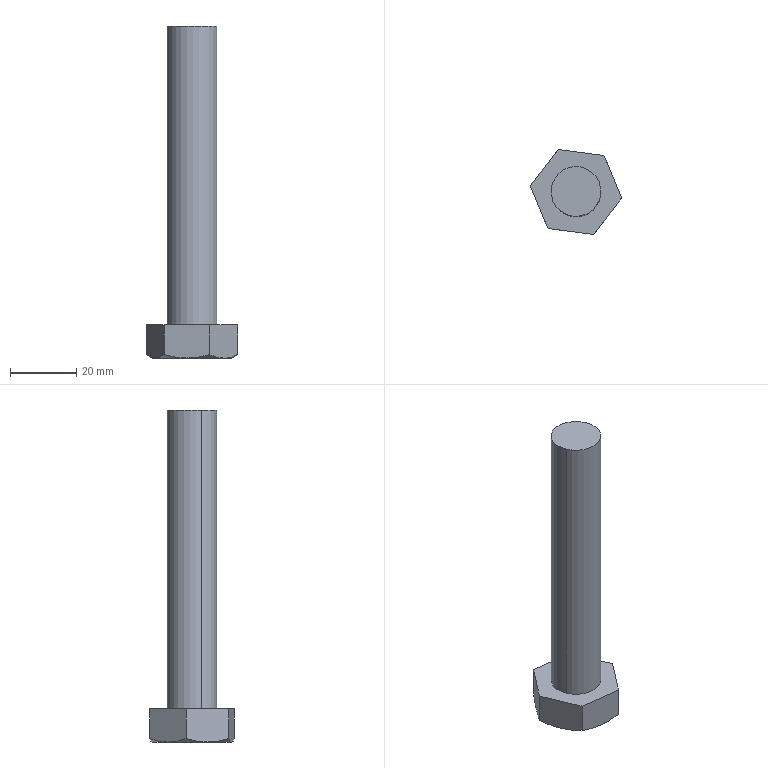Part | SolidWorks | features BaseBody 1 | 1 solid | 17 faces | box 27.477 x 25.599 x 100 mm | volume 20878 mm3 | plane 9 | cone 6 | cylinder 2 | commonest cylinder face diameters 15 x2
STEP:
#1=CARTESIAN_POINT('',(263.515,1086.351,-654.893));
#2=VERTEX_POINT('',#1);
#3=CARTESIAN_POINT('',(253.992,1093.652,-654.893));
#4=VERTEX_POINT('',#3);
#5=CARTESIAN_POINT('',(265.077,1098.249,-654.893));
#6=DIRECTION('',(0.,0.,-1.));
#7=DIRECTION('',(-0.9237,-0.383,0.));
#8=AXIS2_PLACEMENT_3D('',#5,#6,#7);
#9=CIRCLE('',#8,12.);
#10=EDGE_CURVE('',#2,#4,#9,.T.);
#11=ORIENTED_EDGE('',*,*,#10,.T.);
#12=CARTESIAN_POINT('',(255.554,1105.55,-654.893));
#13=VERTEX_POINT('',#12);
#14=CARTESIAN_POINT('',(265.077,1098.249,-654.893));
#15=DIRECTION('',(0.,0.,-1.));
#16=DIRECTION('',(-0.9237,-0.383,0.));
#17=AXIS2_PLACEMENT_3D('',#14,#15,#16);
#18=CIRCLE('',#17,12.);
#19=EDGE_CURVE('',#4,#13,#18,.T.);
#20=ORIENTED_EDGE('',*,*,#19,.T.);
#21=CARTESIAN_POINT('',(266.639,1110.147,-654.893));
#22=VERTEX_POINT('',#21);
#23=CARTESIAN_POINT('',(265.077,1098.249,-654.893));
#24=DIRECTION('',(0.,0.,-1.));
#25=DIRECTION('',(-0.9237,-0.383,0.));
#26=AXIS2_PLACEMENT_3D('',#23,#24,#25);
#27=CIRCLE('',#26,12.);
#28=EDGE_CURVE('',#13,#22,#27,.T.);
#29=ORIENTED_EDGE('',*,*,#28,.T.);
#30=CARTESIAN_POINT('',(276.162,1102.846,-654.893));
#31=VERTEX_POINT('',#30);
#32=CARTESIAN_POINT('',(265.077,1098.249,-654.893));
#33=DIRECTION('',(0.,0.,-1.));
#34=DIRECTION('',(-0.9237,-0.383,0.));
#35=AXIS2_PLACEMENT_3D('',#32,#33,#34);
#36=CIRCLE('',#35,12.);
#37=EDGE_CURVE('',#22,#31,#36,.T.);
#38=ORIENTED_EDGE('',*,*,#37,.T.);
#39=CARTESIAN_POINT('',(274.6,1090.948,-654.893));
#40=VERTEX_POINT('',#39);
#41=CARTESIAN_POINT('',(265.077,1098.249,-654.893));
#42=DIRECTION('',(0.,0.,-1.));
#43=DIRECTION('',(-0.9237,-0.383,0.));
#44=AXIS2_PLACEMENT_3D('',#41,#42,#43);
#45=CIRCLE('',#44,12.);
#46=EDGE_CURVE('',#31,#40,#45,.T.);
#47=ORIENTED_EDGE('',*,*,#46,.T.);
#48=CARTESIAN_POINT('',(265.077,1098.249,-654.893));
#49=DIRECTION('',(0.,0.,-1.));
#50=DIRECTION('',(-0.9237,-0.383,0.));
#51=AXIS2_PLACEMENT_3D('',#48,#49,#50);
#52=CIRCLE('',#51,12.);
#53=EDGE_CURVE('',#40,#2,#52,.T.);
#54=ORIENTED_EDGE('',*,*,#53,.T.);
#55=EDGE_LOOP('',(#11,#20,#29,#38,#47,#54));
#56=FACE_OUTER_BOUND('',#55,.T.);
#57=CARTESIAN_POINT('',(259.769,1111.048,-654.893));
#58=DIRECTION('',(0.,0.,-1.));
#59=DIRECTION('',(0.,-1.,0.));
#60=AXIS2_PLACEMENT_3D('',#57,#58,#59);
#61=PLANE('',#60);
#62=ADVANCED_FACE('',(#56),#61,.T.);
#63=CARTESIAN_POINT('',(251.338,1100.052,-653.822));
#64=VERTEX_POINT('',#63);
#65=CARTESIAN_POINT('',(251.338,1100.052,-653.822));
#66=CARTESIAN_POINT('',(251.697,1100.52,-653.992));
#67=CARTESIAN_POINT('',(252.049,1100.978,-654.142));
#68=CARTESIAN_POINT('',(252.568,1101.655,-654.338));
#69=CARTESIAN_POINT('',(252.74,1101.88,-654.398));
#70=CARTESIAN_POINT('',(252.996,1102.215,-654.481));
#71=CARTESIAN_POINT('',(253.125,1102.382,-654.521));
#72=CARTESIAN_POINT('',(253.274,1102.576,-654.564));
#73=CARTESIAN_POINT('',(253.338,1102.66,-654.581));
#74=CARTESIAN_POINT('',(253.38,1102.715,-654.593));
#75=CARTESIAN_POINT('',(253.401,1102.742,-654.598));
#76=CARTESIAN_POINT('',(253.601,1103.003,-654.652));
#77=CARTESIAN_POINT('',(253.777,1103.233,-654.693));
#78=CARTESIAN_POINT('',(254.042,1103.578,-654.747));
#79=CARTESIAN_POINT('',(254.174,1103.75,-654.771));
#80=CARTESIAN_POINT('',(254.306,1103.922,-654.793));
#81=CARTESIAN_POINT('',(254.394,1104.037,-654.806));
#82=CARTESIAN_POINT('',(254.437,1104.093,-654.813));
#83=CARTESIAN_POINT('',(254.841,1104.621,-654.869));
#84=CARTESIAN_POINT('',(255.196,1105.084,-654.893));
#85=CARTESIAN_POINT('',(255.554,1105.55,-654.893));
#86=B_SPLINE_CURVE_WITH_KNOTS('',3,(#65,#66,#67,#68,#69,#70,#71,#72,#73,#74,#75,#76,#77,#78,#79,#80,#81,#82,#83,#84,#85),.UNSPECIFIED.,.F.,.F.,(4,2,2,1,1,2,2,2,1,2,2,4),(0.,0.25,0.375,0.4375,0.4688,0.4844,0.5,0.625,0.6875,0.7188,0.75,1.),.UNSPECIFIED.);
#87=EDGE_CURVE('',#64,#13,#86,.T.);
#88=ORIENTED_EDGE('',*,*,#87,.T.);
#89=ORIENTED_EDGE('',*,*,#19,.F.);
#90=CARTESIAN_POINT('',(253.992,1093.652,-654.893));
#91=CARTESIAN_POINT('',(253.88,1093.924,-654.893));
#92=CARTESIAN_POINT('',(253.767,1094.194,-654.887));
#93=CARTESIAN_POINT('',(253.599,1094.6,-654.869));
#94=CARTESIAN_POINT('',(253.543,1094.736,-654.861));
#95=CARTESIAN_POINT('',(253.458,1094.94,-654.847));
#96=CARTESIAN_POINT('',(253.43,1095.007,-654.842));
#97=CARTESIAN_POINT('',(253.374,1095.144,-654.831));
#98=CARTESIAN_POINT('',(253.345,1095.213,-654.825));
#99=CARTESIAN_POINT('',(253.206,1095.547,-654.795));
#100=CARTESIAN_POINT('',(253.096,1095.814,-654.765));
#101=CARTESIAN_POINT('',(252.929,1096.215,-654.711));
#102=CARTESIAN_POINT('',(252.846,1096.416,-654.682));
#103=CARTESIAN_POINT('',(252.748,1096.652,-654.644));
#104=CARTESIAN_POINT('',(252.707,1096.753,-654.627));
#105=CARTESIAN_POINT('',(252.679,1096.82,-654.616));
#106=CARTESIAN_POINT('',(252.664,1096.855,-654.61));
#107=CARTESIAN_POINT('',(252.222,1097.922,-654.423));
#108=CARTESIAN_POINT('',(251.79,1098.962,-654.162));
#109=CARTESIAN_POINT('',(251.338,1100.052,-653.822));
#110=B_SPLINE_CURVE_WITH_KNOTS('',3,(#90,#91,#92,#93,#94,#95,#96,#97,#98,#99,#100,#101,#102,#103,#104,#105,#106,#107,#108,#109),.UNSPECIFIED.,.F.,.F.,(4,2,2,2,2,2,1,1,2,2,4),(0.,0.125,0.1875,0.2188,0.25,0.375,0.4375,0.4688,0.4844,0.5,1.),.UNSPECIFIED.);
#111=EDGE_CURVE('',#4,#64,#110,.T.);
#112=ORIENTED_EDGE('',*,*,#111,.T.);
#113=EDGE_LOOP('',(#88,#89,#112));
#114=FACE_OUTER_BOUND('',#113,.T.);
#115=CARTESIAN_POINT('',(265.077,1098.249,-654.893));
#116=DIRECTION('',(0.,0.,1.));
#117=DIRECTION('',(0.9237,0.383,0.));
#118=AXIS2_PLACEMENT_3D('',#115,#116,#117);
#119=CONICAL_SURFACE('',#118,12.,1.047);
#120=ADVANCED_FACE('',(#114),#119,.T.);
#121=CARTESIAN_POINT('',(259.769,1111.048,-653.822));
#122=VERTEX_POINT('',#121);
#123=CARTESIAN_POINT('',(255.554,1105.55,-654.893));
#124=CARTESIAN_POINT('',(255.733,1105.784,-654.893));
#125=CARTESIAN_POINT('',(255.911,1106.016,-654.887));
#126=CARTESIAN_POINT('',(256.178,1106.365,-654.869));
#127=CARTESIAN_POINT('',(256.312,1106.539,-654.857));
#128=CARTESIAN_POINT('',(256.446,1106.715,-654.842));
#129=CARTESIAN_POINT('',(256.536,1106.832,-654.831));
#130=CARTESIAN_POINT('',(256.582,1106.891,-654.825));
#131=CARTESIAN_POINT('',(256.802,1107.178,-654.795));
#132=CARTESIAN_POINT('',(256.978,1107.408,-654.765));
#133=CARTESIAN_POINT('',(257.242,1107.752,-654.711));
#134=CARTESIAN_POINT('',(257.374,1107.925,-654.682));
#135=CARTESIAN_POINT('',(257.529,1108.127,-654.644));
#136=CARTESIAN_POINT('',(257.596,1108.214,-654.627));
#137=CARTESIAN_POINT('',(257.64,1108.272,-654.616));
#138=CARTESIAN_POINT('',(257.663,1108.302,-654.61));
#139=CARTESIAN_POINT('',(258.366,1109.218,-654.423));
#140=CARTESIAN_POINT('',(259.051,1110.112,-654.162));
#141=CARTESIAN_POINT('',(259.769,1111.048,-653.822));
#142=B_SPLINE_CURVE_WITH_KNOTS('',3,(#123,#124,#125,#126,#127,#128,#129,#130,#131,#132,#133,#134,#135,#136,#137,#138,#139,#140,#141),.UNSPECIFIED.,.F.,.F.,(4,2,1,2,2,2,1,1,2,2,4),(0.,0.125,0.1875,0.2187,0.25,0.375,0.4375,0.4687,0.4844,0.5,1.),.UNSPECIFIED.);
#143=EDGE_CURVE('',#13,#122,#142,.T.);
#144=ORIENTED_EDGE('',*,*,#143,.T.);
#145=CARTESIAN_POINT('',(259.769,1111.048,-653.822));
#146=CARTESIAN_POINT('',(260.354,1110.972,-653.992));
#147=CARTESIAN_POINT('',(260.926,1110.896,-654.142));
#148=CARTESIAN_POINT('',(261.773,1110.785,-654.338));
#149=CARTESIAN_POINT('',(262.053,1110.749,-654.398));
#150=CARTESIAN_POINT('',(262.471,1110.694,-654.481));
#151=CARTESIAN_POINT('',(262.68,1110.666,-654.521));
#152=CARTESIAN_POINT('',(262.923,1110.635,-654.564));
#153=CARTESIAN_POINT('',(263.027,1110.621,-654.581));
#154=CARTESIAN_POINT('',(263.097,1110.612,-654.593));
#155=CARTESIAN_POINT('',(263.13,1110.607,-654.598));
#156=CARTESIAN_POINT('',(263.456,1110.565,-654.652));
#157=CARTESIAN_POINT('',(263.744,1110.527,-654.693));
#158=CARTESIAN_POINT('',(264.175,1110.47,-654.747));
#159=CARTESIAN_POINT('',(264.318,1110.452,-654.763));
#160=CARTESIAN_POINT('',(264.533,1110.423,-654.786));
#161=CARTESIAN_POINT('',(264.605,1110.414,-654.793));
#162=CARTESIAN_POINT('',(264.748,1110.395,-654.806));
#163=CARTESIAN_POINT('',(264.818,1110.386,-654.813));
#164=CARTESIAN_POINT('',(265.477,1110.299,-654.869));
#165=CARTESIAN_POINT('',(266.056,1110.223,-654.893));
#166=CARTESIAN_POINT('',(266.639,1110.147,-654.893));
#167=B_SPLINE_CURVE_WITH_KNOTS('',3,(#145,#146,#147,#148,#149,#150,#151,#152,#153,#154,#155,#156,#157,#158,#159,#160,#161,#162,#163,#164,#165,#166),.UNSPECIFIED.,.F.,.F.,(4,2,2,1,1,2,2,2,2,2,2,4),(0.,0.25,0.375,0.4375,0.4688,0.4844,0.5,0.625,0.6875,0.7188,0.75,1.),.UNSPECIFIED.);
#168=EDGE_CURVE('',#122,#22,#167,.T.);
#169=ORIENTED_EDGE('',*,*,#168,.T.);
#170=ORIENTED_EDGE('',*,*,#28,.F.);
#171=EDGE_LOOP('',(#144,#169,#170));
#172=FACE_OUTER_BOUND('',#171,.T.);
#173=CARTESIAN_POINT('',(265.077,1098.249,-654.893));
#174=DIRECTION('',(0.,0.,1.));
#175=DIRECTION('',(0.9237,0.383,0.));
#176=AXIS2_PLACEMENT_3D('',#173,#174,#175);
#177=CONICAL_SURFACE('',#176,12.,1.047);
#178=ADVANCED_FACE('',(#172),#177,.T.);
#179=CARTESIAN_POINT('',(273.508,1109.245,-653.822));
#180=VERTEX_POINT('',#179);
#181=CARTESIAN_POINT('',(266.639,1110.147,-654.893));
#182=CARTESIAN_POINT('',(266.93,1110.109,-654.893));
#183=CARTESIAN_POINT('',(267.22,1110.071,-654.887));
#184=CARTESIAN_POINT('',(267.656,1110.013,-654.869));
#185=CARTESIAN_POINT('',(267.802,1109.994,-654.861));
#186=CARTESIAN_POINT('',(268.02,1109.966,-654.847));
#187=CARTESIAN_POINT('',(268.093,1109.956,-654.842));
#188=CARTESIAN_POINT('',(268.239,1109.937,-654.831));
#189=CARTESIAN_POINT('',(268.314,1109.927,-654.825));
#190=CARTESIAN_POINT('',(268.672,1109.88,-654.795));
#191=CARTESIAN_POINT('',(268.959,1109.842,-654.765));
#192=CARTESIAN_POINT('',(269.39,1109.786,-654.711));
#193=CARTESIAN_POINT('',(269.605,1109.758,-654.682));
#194=CARTESIAN_POINT('',(269.858,1109.724,-654.644));
#195=CARTESIAN_POINT('',(269.966,1109.71,-654.627));
#196=CARTESIAN_POINT('',(270.039,1109.701,-654.616));
#197=CARTESIAN_POINT('',(270.076,1109.696,-654.61));
#198=CARTESIAN_POINT('',(271.221,1109.545,-654.423));
#199=CARTESIAN_POINT('',(272.338,1109.399,-654.162));
#200=CARTESIAN_POINT('',(273.508,1109.245,-653.822));
#201=B_SPLINE_CURVE_WITH_KNOTS('',3,(#181,#182,#183,#184,#185,#186,#187,#188,#189,#190,#191,#192,#193,#194,#195,#196,#197,#198,#199,#200),.UNSPECIFIED.,.F.,.F.,(4,2,2,2,2,2,1,1,2,2,4),(0.,0.125,0.1875,0.2187,0.25,0.375,0.4375,0.4687,0.4844,0.5,1.),.UNSPECIFIED.);
#202=EDGE_CURVE('',#22,#180,#201,.T.);
#203=ORIENTED_EDGE('',*,*,#202,.T.);
#204=CARTESIAN_POINT('',(273.508,1109.245,-653.822));
#205=CARTESIAN_POINT('',(273.734,1108.7,-653.992));
#206=CARTESIAN_POINT('',(273.955,1108.167,-654.142));
#207=CARTESIAN_POINT('',(274.281,1107.379,-654.338));
#208=CARTESIAN_POINT('',(274.39,1107.118,-654.398));
#209=CARTESIAN_POINT('',(274.552,1106.728,-654.481));
#210=CARTESIAN_POINT('',(274.632,1106.534,-654.521));
#211=CARTESIAN_POINT('',(274.726,1106.307,-654.564));
#212=CARTESIAN_POINT('',(274.766,1106.21,-654.581));
#213=CARTESIAN_POINT('',(274.793,1106.145,-654.593));
#214=CARTESIAN_POINT('',(274.806,1106.114,-654.598));
#215=CARTESIAN_POINT('',(274.932,1105.811,-654.652));
#216=CARTESIAN_POINT('',(275.043,1105.542,-654.693));
#217=CARTESIAN_POINT('',(275.21,1105.141,-654.747));
#218=CARTESIAN_POINT('',(275.293,1104.941,-654.771));
#219=CARTESIAN_POINT('',(275.376,1104.74,-654.793));
#220=CARTESIAN_POINT('',(275.431,1104.607,-654.806));
#221=CARTESIAN_POINT('',(275.459,1104.541,-654.813));
#222=CARTESIAN_POINT('',(275.713,1103.927,-654.869));
#223=CARTESIAN_POINT('',(275.936,1103.388,-654.893));
#224=CARTESIAN_POINT('',(276.162,1102.846,-654.893));
#225=B_SPLINE_CURVE_WITH_KNOTS('',3,(#204,#205,#206,#207,#208,#209,#210,#211,#212,#213,#214,#215,#216,#217,#218,#219,#220,#221,#222,#223,#224),.UNSPECIFIED.,.F.,.F.,(4,2,2,1,1,2,2,2,1,2,2,4),(0.,0.25,0.375,0.4375,0.4688,0.4844,0.5,0.625,0.6875,0.7188,0.75,1.),.UNSPECIFIED.);
#226=EDGE_CURVE('',#180,#31,#225,.T.);
#227=ORIENTED_EDGE('',*,*,#226,.T.);
#228=ORIENTED_EDGE('',*,*,#37,.F.);
#229=EDGE_LOOP('',(#203,#227,#228));
#230=FACE_OUTER_BOUND('',#229,.T.);
#231=CARTESIAN_POINT('',(265.077,1098.249,-654.893));
#232=DIRECTION('',(0.,0.,1.));
#233=DIRECTION('',(0.9237,0.383,0.));
#234=AXIS2_PLACEMENT_3D('',#231,#232,#233);
#235=CONICAL_SURFACE('',#234,12.,1.047);
#236=ADVANCED_FACE('',(#230),#235,.T.);
#237=CARTESIAN_POINT('',(278.815,1096.446,-653.822));
#238=VERTEX_POINT('',#237);
#239=CARTESIAN_POINT('',(276.162,1102.846,-654.893));
#240=CARTESIAN_POINT('',(276.274,1102.574,-654.893));
#241=CARTESIAN_POINT('',(276.386,1102.304,-654.887));
#242=CARTESIAN_POINT('',(276.555,1101.897,-654.869));
#243=CARTESIAN_POINT('',(276.611,1101.762,-654.861));
#244=CARTESIAN_POINT('',(276.695,1101.558,-654.847));
#245=CARTESIAN_POINT('',(276.724,1101.49,-654.842));
#246=CARTESIAN_POINT('',(276.78,1101.354,-654.831));
#247=CARTESIAN_POINT('',(276.809,1101.285,-654.825));
#248=CARTESIAN_POINT('',(276.948,1100.951,-654.795));
#249=CARTESIAN_POINT('',(277.058,1100.684,-654.765));
#250=CARTESIAN_POINT('',(277.224,1100.282,-654.711));
#251=CARTESIAN_POINT('',(277.308,1100.082,-654.682));
#252=CARTESIAN_POINT('',(277.405,1099.846,-654.644));
#253=CARTESIAN_POINT('',(277.447,1099.745,-654.627));
#254=CARTESIAN_POINT('',(277.475,1099.678,-654.616));
#255=CARTESIAN_POINT('',(277.49,1099.643,-654.61));
#256=CARTESIAN_POINT('',(277.932,1098.576,-654.423));
#257=CARTESIAN_POINT('',(278.363,1097.536,-654.162));
#258=CARTESIAN_POINT('',(278.815,1096.446,-653.822));
#259=B_SPLINE_CURVE_WITH_KNOTS('',3,(#239,#240,#241,#242,#243,#244,#245,#246,#247,#248,#249,#250,#251,#252,#253,#254,#255,#256,#257,#258),.UNSPECIFIED.,.F.,.F.,(4,2,2,2,2,2,1,1,2,2,4),(0.,0.125,0.1875,0.2188,0.25,0.375,0.4375,0.4688,0.4844,0.5,1.),.UNSPECIFIED.);
#260=EDGE_CURVE('',#31,#238,#259,.T.);
#261=ORIENTED_EDGE('',*,*,#260,.T.);
#262=CARTESIAN_POINT('',(278.815,1096.446,-653.822));
#263=CARTESIAN_POINT('',(278.456,1095.977,-653.992));
#264=CARTESIAN_POINT('',(278.105,1095.52,-654.142));
#265=CARTESIAN_POINT('',(277.586,1094.842,-654.338));
#266=CARTESIAN_POINT('',(277.414,1094.618,-654.398));
#267=CARTESIAN_POINT('',(277.157,1094.283,-654.481));
#268=CARTESIAN_POINT('',(277.029,1094.116,-654.521));
#269=CARTESIAN_POINT('',(276.88,1093.921,-654.564));
#270=CARTESIAN_POINT('',(276.816,1093.838,-654.581));
#271=CARTESIAN_POINT('',(276.774,1093.783,-654.593));
#272=CARTESIAN_POINT('',(276.753,1093.756,-654.598));
#273=CARTESIAN_POINT('',(276.553,1093.495,-654.652));
#274=CARTESIAN_POINT('',(276.376,1093.265,-654.693));
#275=CARTESIAN_POINT('',(276.112,1092.92,-654.747));
#276=CARTESIAN_POINT('',(275.98,1092.748,-654.771));
#277=CARTESIAN_POINT('',(275.848,1092.575,-654.793));
#278=CARTESIAN_POINT('',(275.76,1092.461,-654.806));
#279=CARTESIAN_POINT('',(275.717,1092.404,-654.813));
#280=CARTESIAN_POINT('',(275.313,1091.877,-654.869));
#281=CARTESIAN_POINT('',(274.958,1091.414,-654.893));
#282=CARTESIAN_POINT('',(274.6,1090.948,-654.893));
#283=B_SPLINE_CURVE_WITH_KNOTS('',3,(#262,#263,#264,#265,#266,#267,#268,#269,#270,#271,#272,#273,#274,#275,#276,#277,#278,#279,#280,#281,#282),.UNSPECIFIED.,.F.,.F.,(4,2,2,1,1,2,2,2,1,2,2,4),(0.,0.25,0.375,0.4375,0.4688,0.4844,0.5,0.625,0.6875,0.7187,0.75,1.),.UNSPECIFIED.);
#284=EDGE_CURVE('',#238,#40,#283,.T.);
#285=ORIENTED_EDGE('',*,*,#284,.T.);
#286=ORIENTED_EDGE('',*,*,#46,.F.);
#287=EDGE_LOOP('',(#261,#285,#286));
#288=FACE_OUTER_BOUND('',#287,.T.);
#289=CARTESIAN_POINT('',(265.077,1098.249,-654.893));
#290=DIRECTION('',(0.,0.,1.));
#291=DIRECTION('',(0.9237,0.383,0.));
#292=AXIS2_PLACEMENT_3D('',#289,#290,#291);
#293=CONICAL_SURFACE('',#292,12.,1.047);
#294=ADVANCED_FACE('',(#288),#293,.T.);
#295=CARTESIAN_POINT('',(270.385,1085.449,-653.822));
#296=VERTEX_POINT('',#295);
#297=CARTESIAN_POINT('',(274.6,1090.948,-654.893));
#298=CARTESIAN_POINT('',(274.421,1090.714,-654.893));
#299=CARTESIAN_POINT('',(274.243,1090.482,-654.887));
#300=CARTESIAN_POINT('',(273.976,1090.133,-654.869));
#301=CARTESIAN_POINT('',(273.842,1089.958,-654.857));
#302=CARTESIAN_POINT('',(273.707,1089.783,-654.842));
#303=CARTESIAN_POINT('',(273.618,1089.666,-654.831));
#304=CARTESIAN_POINT('',(273.572,1089.607,-654.825));
#305=CARTESIAN_POINT('',(273.352,1089.32,-654.795));
#306=CARTESIAN_POINT('',(273.176,1089.09,-654.765));
#307=CARTESIAN_POINT('',(272.912,1088.746,-654.711));
#308=CARTESIAN_POINT('',(272.779,1088.573,-654.682));
#309=CARTESIAN_POINT('',(272.624,1088.371,-654.644));
#310=CARTESIAN_POINT('',(272.558,1088.284,-654.627));
#311=CARTESIAN_POINT('',(272.514,1088.226,-654.616));
#312=CARTESIAN_POINT('',(272.49,1088.196,-654.61));
#313=CARTESIAN_POINT('',(271.788,1087.28,-654.423));
#314=CARTESIAN_POINT('',(271.103,1086.386,-654.162));
#315=CARTESIAN_POINT('',(270.385,1085.449,-653.822));
#316=B_SPLINE_CURVE_WITH_KNOTS('',3,(#297,#298,#299,#300,#301,#302,#303,#304,#305,#306,#307,#308,#309,#310,#311,#312,#313,#314,#315),.UNSPECIFIED.,.F.,.F.,(4,2,1,2,2,2,1,1,2,2,4),(0.,0.125,0.1875,0.2188,0.25,0.375,0.4375,0.4688,0.4844,0.5,1.),.UNSPECIFIED.);
#317=EDGE_CURVE('',#40,#296,#316,.T.);
#318=ORIENTED_EDGE('',*,*,#317,.T.);
#319=CARTESIAN_POINT('',(270.385,1085.449,-653.822));
#320=CARTESIAN_POINT('',(269.799,1085.526,-653.992));
#321=CARTESIAN_POINT('',(269.227,1085.602,-654.142));
#322=CARTESIAN_POINT('',(268.381,1085.713,-654.338));
#323=CARTESIAN_POINT('',(268.101,1085.749,-654.398));
#324=CARTESIAN_POINT('',(267.683,1085.804,-654.481));
#325=CARTESIAN_POINT('',(267.474,1085.831,-654.521));
#326=CARTESIAN_POINT('',(267.231,1085.863,-654.564));
#327=CARTESIAN_POINT('',(267.127,1085.877,-654.581));
#328=CARTESIAN_POINT('',(267.057,1085.886,-654.593));
#329=CARTESIAN_POINT('',(267.024,1085.89,-654.598));
#330=CARTESIAN_POINT('',(266.698,1085.933,-654.652));
#331=CARTESIAN_POINT('',(266.41,1085.971,-654.693));
#332=CARTESIAN_POINT('',(265.979,1086.028,-654.747));
#333=CARTESIAN_POINT('',(265.836,1086.046,-654.763));
#334=CARTESIAN_POINT('',(265.621,1086.075,-654.786));
#335=CARTESIAN_POINT('',(265.549,1086.084,-654.793));
#336=CARTESIAN_POINT('',(265.406,1086.103,-654.806));
#337=CARTESIAN_POINT('',(265.336,1086.112,-654.813));
#338=CARTESIAN_POINT('',(264.676,1086.198,-654.869));
#339=CARTESIAN_POINT('',(264.098,1086.275,-654.893));
#340=CARTESIAN_POINT('',(263.515,1086.351,-654.893));
#341=B_SPLINE_CURVE_WITH_KNOTS('',3,(#319,#320,#321,#322,#323,#324,#325,#326,#327,#328,#329,#330,#331,#332,#333,#334,#335,#336,#337,#338,#339,#340),.UNSPECIFIED.,.F.,.F.,(4,2,2,1,1,2,2,2,2,2,2,4),(0.,0.25,0.375,0.4375,0.4688,0.4844,0.5,0.625,0.6875,0.7188,0.75,1.),.UNSPECIFIED.);
#342=EDGE_CURVE('',#296,#2,#341,.T.);
#343=ORIENTED_EDGE('',*,*,#342,.T.);
#344=ORIENTED_EDGE('',*,*,#53,.F.);
#345=EDGE_LOOP('',(#318,#343,#344));
#346=FACE_OUTER_BOUND('',#345,.T.);
#347=CARTESIAN_POINT('',(265.077,1098.249,-654.893));
#348=DIRECTION('',(0.,0.,1.));
#349=DIRECTION('',(0.9237,0.383,0.));
#350=AXIS2_PLACEMENT_3D('',#347,#348,#349);
#351=CONICAL_SURFACE('',#350,12.,1.047);
#352=ADVANCED_FACE('',(#346),#351,.T.);
#353=CARTESIAN_POINT('',(256.646,1087.253,-653.822));
#354=VERTEX_POINT('',#353);
#355=CARTESIAN_POINT('',(263.515,1086.351,-654.893));
#356=CARTESIAN_POINT('',(263.224,1086.389,-654.893));
#357=CARTESIAN_POINT('',(262.934,1086.427,-654.887));
#358=CARTESIAN_POINT('',(262.498,1086.485,-654.869));
#359=CARTESIAN_POINT('',(262.352,1086.504,-654.861));
#360=CARTESIAN_POINT('',(262.134,1086.532,-654.847));
#361=CARTESIAN_POINT('',(262.061,1086.542,-654.842));
#362=CARTESIAN_POINT('',(261.915,1086.561,-654.831));
#363=CARTESIAN_POINT('',(261.84,1086.571,-654.825));
#364=CARTESIAN_POINT('',(261.481,1086.618,-654.795));
#365=CARTESIAN_POINT('',(261.195,1086.656,-654.765));
#366=CARTESIAN_POINT('',(260.764,1086.712,-654.711));
#367=CARTESIAN_POINT('',(260.549,1086.74,-654.682));
#368=CARTESIAN_POINT('',(260.296,1086.774,-654.644));
#369=CARTESIAN_POINT('',(260.188,1086.788,-654.627));
#370=CARTESIAN_POINT('',(260.115,1086.797,-654.616));
#371=CARTESIAN_POINT('',(260.077,1086.802,-654.61));
#372=CARTESIAN_POINT('',(258.933,1086.952,-654.423));
#373=CARTESIAN_POINT('',(257.816,1087.099,-654.162));
#374=CARTESIAN_POINT('',(256.646,1087.253,-653.822));
#375=B_SPLINE_CURVE_WITH_KNOTS('',3,(#355,#356,#357,#358,#359,#360,#361,#362,#363,#364,#365,#366,#367,#368,#369,#370,#371,#372,#373,#374),.UNSPECIFIED.,.F.,.F.,(4,2,2,2,2,2,1,1,2,2,4),(0.,0.125,0.1875,0.2188,0.25,0.375,0.4375,0.4688,0.4844,0.5,1.),.UNSPECIFIED.);
#376=EDGE_CURVE('',#2,#354,#375,.T.);
#377=ORIENTED_EDGE('',*,*,#376,.T.);
#378=CARTESIAN_POINT('',(256.646,1087.253,-653.822));
#379=CARTESIAN_POINT('',(256.42,1087.798,-653.992));
#380=CARTESIAN_POINT('',(256.199,1088.331,-654.142));
#381=CARTESIAN_POINT('',(255.872,1089.119,-654.338));
#382=CARTESIAN_POINT('',(255.764,1089.38,-654.398));
#383=CARTESIAN_POINT('',(255.602,1089.77,-654.481));
#384=CARTESIAN_POINT('',(255.522,1089.964,-654.521));
#385=CARTESIAN_POINT('',(255.428,1090.191,-654.564));
#386=CARTESIAN_POINT('',(255.387,1090.288,-654.581));
#387=CARTESIAN_POINT('',(255.361,1090.353,-654.593));
#388=CARTESIAN_POINT('',(255.348,1090.383,-654.598));
#389=CARTESIAN_POINT('',(255.222,1090.687,-654.652));
#390=CARTESIAN_POINT('',(255.111,1090.955,-654.693));
#391=CARTESIAN_POINT('',(254.944,1091.357,-654.747));
#392=CARTESIAN_POINT('',(254.861,1091.557,-654.771));
#393=CARTESIAN_POINT('',(254.778,1091.757,-654.793));
#394=CARTESIAN_POINT('',(254.722,1091.891,-654.806));
#395=CARTESIAN_POINT('',(254.695,1091.956,-654.813));
#396=CARTESIAN_POINT('',(254.441,1092.571,-654.869));
#397=CARTESIAN_POINT('',(254.217,1093.109,-654.893));
#398=CARTESIAN_POINT('',(253.992,1093.652,-654.893));
#399=B_SPLINE_CURVE_WITH_KNOTS('',3,(#378,#379,#380,#381,#382,#383,#384,#385,#386,#387,#388,#389,#390,#391,#392,#393,#394,#395,#396,#397,#398),.UNSPECIFIED.,.F.,.F.,(4,2,2,1,1,2,2,2,1,2,2,4),(0.,0.25,0.375,0.4375,0.4688,0.4844,0.5,0.625,0.6875,0.7187,0.75,1.),.UNSPECIFIED.);
#400=EDGE_CURVE('',#354,#4,#399,.T.);
#401=ORIENTED_EDGE('',*,*,#400,.T.);
#402=ORIENTED_EDGE('',*,*,#10,.F.);
#403=EDGE_LOOP('',(#377,#401,#402));
#404=FACE_OUTER_BOUND('',#403,.T.);
#405=CARTESIAN_POINT('',(265.077,1098.249,-654.893));
#406=DIRECTION('',(0.,0.,1.));
#407=DIRECTION('',(0.9237,0.383,0.));
#408=AXIS2_PLACEMENT_3D('',#405,#406,#407);
#409=CONICAL_SURFACE('',#408,12.,1.047);
#410=ADVANCED_FACE('',(#404),#409,.T.);
#411=CARTESIAN_POINT('',(272.005,1101.122,-644.893));
#412=VERTEX_POINT('',#411);
#413=CARTESIAN_POINT('',(258.149,1095.376,-644.893));
#414=VERTEX_POINT('',#413);
#415=CARTESIAN_POINT('',(265.077,1098.249,-644.893));
#416=DIRECTION('',(0.,0.,-1.));
#417=DIRECTION('',(-0.9237,-0.383,0.));
#418=AXIS2_PLACEMENT_3D('',#415,#416,#417);
#419=CIRCLE('',#418,7.5);
#420=EDGE_CURVE('',#412,#414,#419,.T.);
#421=ORIENTED_EDGE('',*,*,#420,.T.);
#422=CARTESIAN_POINT('',(265.077,1098.249,-644.893));
#423=DIRECTION('',(0.,0.,-1.));
#424=DIRECTION('',(-0.9237,-0.383,0.));
#425=AXIS2_PLACEMENT_3D('',#422,#423,#424);
#426=CIRCLE('',#425,7.5);
#427=EDGE_CURVE('',#414,#412,#426,.T.);
#428=ORIENTED_EDGE('',*,*,#427,.T.);
#429=EDGE_LOOP('',(#421,#428));
#430=FACE_BOUND('',#429,.T.);
#431=CARTESIAN_POINT('',(251.338,1100.052,-644.893));
#432=VERTEX_POINT('',#431);
#433=CARTESIAN_POINT('',(259.769,1111.048,-644.893));
#434=VERTEX_POINT('',#433);
#435=CARTESIAN_POINT('',(251.338,1100.052,-644.893));
#436=DIRECTION('',(0.6084,0.7936,0.));
#437=VECTOR('',#436,1000.);
#438=LINE('',#435,#437);
#439=EDGE_CURVE('',#432,#434,#438,.T.);
#440=ORIENTED_EDGE('',*,*,#439,.F.);
#441=CARTESIAN_POINT('',(256.646,1087.253,-644.893));
#442=VERTEX_POINT('',#441);
#443=CARTESIAN_POINT('',(256.646,1087.253,-644.893));
#444=DIRECTION('',(-0.383,0.9237,0.));
#445=VECTOR('',#444,1000.);
#446=LINE('',#443,#445);
#447=EDGE_CURVE('',#442,#432,#446,.T.);
#448=ORIENTED_EDGE('',*,*,#447,.F.);
#449=CARTESIAN_POINT('',(270.385,1085.449,-644.893));
#450=VERTEX_POINT('',#449);
#451=CARTESIAN_POINT('',(270.385,1085.449,-644.893));
#452=DIRECTION('',(-0.9915,0.1301,0.));
#453=VECTOR('',#452,1000.);
#454=LINE('',#451,#453);
#455=EDGE_CURVE('',#450,#442,#454,.T.);
#456=ORIENTED_EDGE('',*,*,#455,.F.);
#457=CARTESIAN_POINT('',(278.815,1096.446,-644.893));
#458=VERTEX_POINT('',#457);
#459=CARTESIAN_POINT('',(278.815,1096.446,-644.893));
#460=DIRECTION('',(-0.6084,-0.7936,0.));
#461=VECTOR('',#460,1000.);
#462=LINE('',#459,#461);
#463=EDGE_CURVE('',#458,#450,#462,.T.);
#464=ORIENTED_EDGE('',*,*,#463,.F.);
#465=CARTESIAN_POINT('',(273.508,1109.245,-644.893));
#466=VERTEX_POINT('',#465);
#467=CARTESIAN_POINT('',(273.508,1109.245,-644.893));
#468=DIRECTION('',(0.383,-0.9237,0.));
#469=VECTOR('',#468,1000.);
#470=LINE('',#467,#469);
#471=EDGE_CURVE('',#466,#458,#470,.T.);
#472=ORIENTED_EDGE('',*,*,#471,.F.);
#473=CARTESIAN_POINT('',(259.769,1111.048,-644.893));
#474=DIRECTION('',(0.9915,-0.1301,0.));
#475=VECTOR('',#474,1000.);
#476=LINE('',#473,#475);
#477=EDGE_CURVE('',#434,#466,#476,.T.);
#478=ORIENTED_EDGE('',*,*,#477,.F.);
#479=EDGE_LOOP('',(#440,#448,#456,#464,#472,#478));
#480=FACE_OUTER_BOUND('',#479,.T.);
#481=CARTESIAN_POINT('',(259.769,1111.048,-644.893));
#482=DIRECTION('',(0.,0.,-1.));
#483=DIRECTION('',(0.,-1.,0.));
#484=AXIS2_PLACEMENT_3D('',#481,#482,#483);
#485=PLANE('',#484);
#486=ADVANCED_FACE('',(#430,#480),#485,.F.);
#487=CARTESIAN_POINT('',(272.005,1101.122,-554.893));
#488=VERTEX_POINT('',#487);
#489=CARTESIAN_POINT('',(258.149,1095.376,-554.893));
#490=VERTEX_POINT('',#489);
#491=CARTESIAN_POINT('',(265.077,1098.249,-554.893));
#492=DIRECTION('',(0.,0.,-1.));
#493=DIRECTION('',(-0.9237,-0.383,0.));
#494=AXIS2_PLACEMENT_3D('',#491,#492,#493);
#495=CIRCLE('',#494,7.5);
#496=EDGE_CURVE('',#488,#490,#495,.T.);
#497=ORIENTED_EDGE('',*,*,#496,.F.);
#498=CARTESIAN_POINT('',(265.077,1098.249,-554.893));
#499=DIRECTION('',(0.,0.,-1.));
#500=DIRECTION('',(-0.9237,-0.383,0.));
#501=AXIS2_PLACEMENT_3D('',#498,#499,#500);
#502=CIRCLE('',#501,7.5);
#503=EDGE_CURVE('',#490,#488,#502,.T.);
#504=ORIENTED_EDGE('',*,*,#503,.F.);
#505=EDGE_LOOP('',(#497,#504));
#506=FACE_OUTER_BOUND('',#505,.T.);
#507=CARTESIAN_POINT('',(265.077,1098.249,-554.893));
#508=DIRECTION('',(0.,0.,-1.));
#509=DIRECTION('',(0.,-1.,0.));
#510=AXIS2_PLACEMENT_3D('',#507,#508,#509);
#511=PLANE('',#510);
#512=ADVANCED_FACE('',(#506),#511,.F.);
#513=CARTESIAN_POINT('',(258.149,1095.376,-644.893));
#514=DIRECTION('',(0.,0.,-1.));
#515=VECTOR('',#514,1000.);
#516=LINE('',#513,#515);
#517=EDGE_CURVE('',#490,#414,#516,.T.);
#518=ORIENTED_EDGE('',*,*,#517,.T.);
#519=ORIENTED_EDGE('',*,*,#420,.F.);
#520=CARTESIAN_POINT('',(272.005,1101.122,-644.893));
#521=DIRECTION('',(0.,0.,-1.));
#522=VECTOR('',#521,1000.);
#523=LINE('',#520,#522);
#524=EDGE_CURVE('',#488,#412,#523,.T.);
#525=ORIENTED_EDGE('',*,*,#524,.F.);
#526=ORIENTED_EDGE('',*,*,#496,.T.);
#527=EDGE_LOOP('',(#518,#519,#525,#526));
#528=FACE_OUTER_BOUND('',#527,.T.);
#529=CARTESIAN_POINT('',(265.077,1098.249,-644.893));
#530=DIRECTION('',(0.,0.,1.));
#531=DIRECTION('',(-0.9237,-0.383,0.));
#532=AXIS2_PLACEMENT_3D('',#529,#530,#531);
#533=CYLINDRICAL_SURFACE('',#532,7.5);
#534=ADVANCED_FACE('',(#528),#533,.T.);
#535=ORIENTED_EDGE('',*,*,#400,.F.);
#536=CARTESIAN_POINT('',(256.646,1087.253,-654.893));
#537=DIRECTION('',(0.,0.,1.));
#538=VECTOR('',#537,1000.);
#539=LINE('',#536,#538);
#540=EDGE_CURVE('',#354,#442,#539,.T.);
#541=ORIENTED_EDGE('',*,*,#540,.T.);
#542=ORIENTED_EDGE('',*,*,#447,.T.);
#543=CARTESIAN_POINT('',(251.338,1100.052,-654.893));
#544=DIRECTION('',(0.,0.,1.));
#545=VECTOR('',#544,1000.);
#546=LINE('',#543,#545);
#547=EDGE_CURVE('',#64,#432,#546,.T.);
#548=ORIENTED_EDGE('',*,*,#547,.F.);
#549=ORIENTED_EDGE('',*,*,#111,.F.);
#550=EDGE_LOOP('',(#535,#541,#542,#548,#549));
#551=FACE_OUTER_BOUND('',#550,.T.);
#552=CARTESIAN_POINT('',(256.646,1087.253,-654.893));
#553=DIRECTION('',(0.9237,0.383,0.));
#554=DIRECTION('',(0.,0.,-1.));
#555=AXIS2_PLACEMENT_3D('',#552,#553,#554);
#556=PLANE('',#555);
#557=ADVANCED_FACE('',(#551),#556,.F.);
#558=ORIENTED_EDGE('',*,*,#342,.F.);
#559=CARTESIAN_POINT('',(270.385,1085.449,-654.893));
#560=DIRECTION('',(0.,0.,1.));
#561=VECTOR('',#560,1000.);
#562=LINE('',#559,#561);
#563=EDGE_CURVE('',#296,#450,#562,.T.);
#564=ORIENTED_EDGE('',*,*,#563,.T.);
#565=ORIENTED_EDGE('',*,*,#455,.T.);
#566=ORIENTED_EDGE('',*,*,#540,.F.);
#567=ORIENTED_EDGE('',*,*,#376,.F.);
#568=EDGE_LOOP('',(#558,#564,#565,#566,#567));
#569=FACE_OUTER_BOUND('',#568,.T.);
#570=CARTESIAN_POINT('',(270.385,1085.449,-654.893));
#571=DIRECTION('',(0.1301,0.9915,0.));
#572=DIRECTION('',(0.,0.,-1.));
#573=AXIS2_PLACEMENT_3D('',#570,#571,#572);
#574=PLANE('',#573);
#575=ADVANCED_FACE('',(#569),#574,.F.);
#576=ORIENTED_EDGE('',*,*,#284,.F.);
#577=CARTESIAN_POINT('',(278.815,1096.446,-654.893));
#578=DIRECTION('',(0.,0.,1.));
#579=VECTOR('',#578,1000.);
#580=LINE('',#577,#579);
#581=EDGE_CURVE('',#238,#458,#580,.T.);
#582=ORIENTED_EDGE('',*,*,#581,.T.);
#583=ORIENTED_EDGE('',*,*,#463,.T.);
#584=ORIENTED_EDGE('',*,*,#563,.F.);
#585=ORIENTED_EDGE('',*,*,#317,.F.);
#586=EDGE_LOOP('',(#576,#582,#583,#584,#585));
#587=FACE_OUTER_BOUND('',#586,.T.);
#588=CARTESIAN_POINT('',(278.815,1096.446,-654.893));
#589=DIRECTION('',(-0.7936,0.6084,0.));
#590=DIRECTION('',(0.,0.,1.));
#591=AXIS2_PLACEMENT_3D('',#588,#589,#590);
#592=PLANE('',#591);
#593=ADVANCED_FACE('',(#587),#592,.F.);
#594=ORIENTED_EDGE('',*,*,#226,.F.);
#595=CARTESIAN_POINT('',(273.508,1109.245,-654.893));
#596=DIRECTION('',(0.,0.,1.));
#597=VECTOR('',#596,1000.);
#598=LINE('',#595,#597);
#599=EDGE_CURVE('',#180,#466,#598,.T.);
#600=ORIENTED_EDGE('',*,*,#599,.T.);
#601=ORIENTED_EDGE('',*,*,#471,.T.);
#602=ORIENTED_EDGE('',*,*,#581,.F.);
#603=ORIENTED_EDGE('',*,*,#260,.F.);
#604=EDGE_LOOP('',(#594,#600,#601,#602,#603));
#605=FACE_OUTER_BOUND('',#604,.T.);
#606=CARTESIAN_POINT('',(273.508,1109.245,-654.893));
#607=DIRECTION('',(-0.9237,-0.383,0.));
#608=DIRECTION('',(-0.383,0.9237,0.));
#609=AXIS2_PLACEMENT_3D('',#606,#607,#608);
#610=PLANE('',#609);
#611=ADVANCED_FACE('',(#605),#610,.F.);
#612=ORIENTED_EDGE('',*,*,#168,.F.);
#613=CARTESIAN_POINT('',(259.769,1111.048,-654.893));
#614=DIRECTION('',(0.,0.,1.));
#615=VECTOR('',#614,1000.);
#616=LINE('',#613,#615);
#617=EDGE_CURVE('',#122,#434,#616,.T.);
#618=ORIENTED_EDGE('',*,*,#617,.T.);
#619=ORIENTED_EDGE('',*,*,#477,.T.);
#620=ORIENTED_EDGE('',*,*,#599,.F.);
#621=ORIENTED_EDGE('',*,*,#202,.F.);
#622=EDGE_LOOP('',(#612,#618,#619,#620,#621));
#623=FACE_OUTER_BOUND('',#622,.T.);
#624=CARTESIAN_POINT('',(259.769,1111.048,-654.893));
#625=DIRECTION('',(-0.1301,-0.9915,0.));
#626=DIRECTION('',(-0.9915,0.1301,0.));
#627=AXIS2_PLACEMENT_3D('',#624,#625,#626);
#628=PLANE('',#627);
#629=ADVANCED_FACE('',(#623),#628,.F.);
#630=ORIENTED_EDGE('',*,*,#87,.F.);
#631=ORIENTED_EDGE('',*,*,#547,.T.);
#632=ORIENTED_EDGE('',*,*,#439,.T.);
#633=ORIENTED_EDGE('',*,*,#617,.F.);
#634=ORIENTED_EDGE('',*,*,#143,.F.);
#635=EDGE_LOOP('',(#630,#631,#632,#633,#634));
#636=FACE_OUTER_BOUND('',#635,.T.);
#637=CARTESIAN_POINT('',(251.338,1100.052,-654.893));
#638=DIRECTION('',(0.7936,-0.6084,0.));
#639=DIRECTION('',(0.,0.,-1.));
#640=AXIS2_PLACEMENT_3D('',#637,#638,#639);
#641=PLANE('',#640);
#642=ADVANCED_FACE('',(#636),#641,.F.);
#643=ORIENTED_EDGE('',*,*,#427,.F.);
#644=ORIENTED_EDGE('',*,*,#517,.F.);
#645=ORIENTED_EDGE('',*,*,#503,.T.);
#646=ORIENTED_EDGE('',*,*,#524,.T.);
#647=EDGE_LOOP('',(#643,#644,#645,#646));
#648=FACE_OUTER_BOUND('',#647,.T.);
#649=CARTESIAN_POINT('',(265.077,1098.249,-644.893));
#650=DIRECTION('',(0.,0.,1.));
#651=DIRECTION('',(-0.9237,-0.383,0.));
#652=AXIS2_PLACEMENT_3D('',#649,#650,#651);
#653=CYLINDRICAL_SURFACE('',#652,7.5);
#654=ADVANCED_FACE('',(#648),#653,.T.);
#655=CLOSED_SHELL('',(#62,#120,#178,#236,#294,#352,#410,#486,#512,#534,#557,#575,#593,#611,#629,#642,#654));
#656=MANIFOLD_SOLID_BREP('',#655);
#657=CARTESIAN_POINT('',(0.,0.,0.));
#658=DIRECTION('',(0.,0.,1.));
#659=DIRECTION('',(1.,0.,0.));
#660=AXIS2_PLACEMENT_3D('',#657,#658,#659);
#661=(LENGTH_UNIT()NAMED_UNIT(*)SI_UNIT(.MILLI.,.METRE.));
#662=UNCERTAINTY_MEASURE_WITH_UNIT(LENGTH_MEASURE(0.00001),#661,'','');
#663=(NAMED_UNIT(*)PLANE_ANGLE_UNIT()SI_UNIT($,.RADIAN.));
#664=(NAMED_UNIT(*)SI_UNIT($,.STERADIAN.)SOLID_ANGLE_UNIT());
#665=(GEOMETRIC_REPRESENTATION_CONTEXT(3)GLOBAL_UNCERTAINTY_ASSIGNED_CONTEXT((#662))GLOBAL_UNIT_ASSIGNED_CONTEXT((#661,#663,#664))REPRESENTATION_CONTEXT('',''));
#666=ADVANCED_BREP_SHAPE_REPRESENTATION('',(#656,#660),#665);